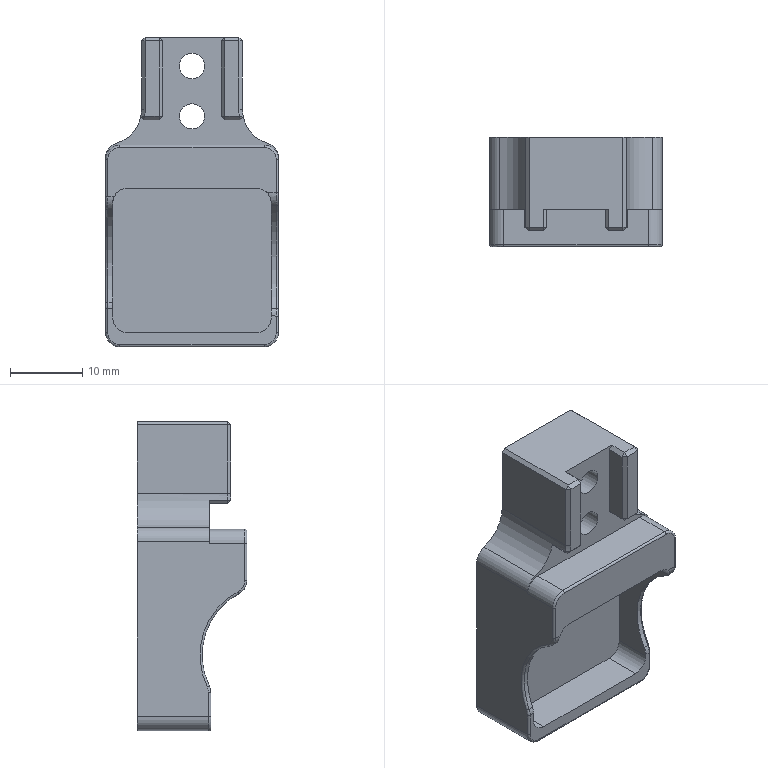CAM job | NX | 3+2 milling, drilling | part box 24 x 15.2 x 43 mm | stock box 25 x 20 x 48 mm
Tools:
number,name,description,diameter,corner_radius,flute_length,length,flutes
3,D3,平底铣刀-粗,3.0,0.0,20.0,75.0,2
6,D6,平底铣刀-粗,6.0,0.0,25.0,75.0,2
9,D10,平底铣刀-粗,10.0,0.0,35.0,75.0,2
17,D3-J,平底铣刀-精,3.0,0.0,50.0,75.0,2
11,D4-J,平底铣刀-精,4.0,0.0,50.0,75.0,2
10,D10-J,平底铣刀-精,10.0,0.0,35.0,75.0,2
1,D80R0.8飞刀,圆鼻刀-粗,80.0,0.8,50.0,75.0,2
2,D6倒角刀,倒角刀,6.0,0.0,3.0,25.0,2
18,R2,圆球刀,4.0,2.0,10.0,50.0,2
17,ZT3.5,钻头,3.5,0.0,35.0,50.0,2
Operations:
program,operation,operation_type,tool,method,geometry_group,spindle_rpm,surface_speed,feed_per_tooth,feed_cut,feed_plunge,cut_length_mm,path_length_mm,cut_time_min,machine_time_min
B,面铣自动飞面开粗一刀_COPY,FaceMilling,D80R0.8飞刀,分层开粗-切深K-步距G,W-B,4500.0,890.615,0.3333,3000.0,100.0,1359.0,2594.622,0.453,0.5766
B,面铣自动飞面精光一刀_COPY,FaceMilling,D80R0.8飞刀,侧刃精光-切深K-步距G,W-B,4500.0,890.615,0.1111,1000.0,100.0,151.0,187.0,0.151,0.1546
B,底壁铣分层开粗-中_COPY_1,VolumeBased25DMillingOperation,D6,分层开粗-切深K-步距G,W-B,8000.0,150.792,0.1875,3000.0,100.0,508.662,593.057,0.1696,0.178
B,型腔铣开粗-中_COPY,CavityMilling,D6,分层开粗-切深K-步距G,W-B,8000.0,150.792,0.1875,3000.0,100.0,6619.858,7262.06,2.207,2.298
B,底壁铣分层开粗-中_COPY,VolumeBased25DMillingOperation,D3,分层开粗-切深K-步距G,W-B,8000.0,100.528,0.125,2000.0,100.0,2179.609,2255.856,1.09,1.097
B,钻倒角_2_1,Operation,D6倒角刀,METHOD,W-B,8000.0,150.796,0.0625,1000.0,0.0,10.1,87.216,0.0101,0.0178
B,钻倒角_2,Operation,D6倒角刀,METHOD,W-B,8000.0,150.796,0.0625,1000.0,0.0,10.1,81.216,0.0101,0.0172
B,平面去毛刺6X45L_COPY,SurfaceContour,D6倒角刀,爬面_倒角-切深0-步距G,W-B,6500.0,122.519,0.1154,1500.0,100.0,80.316,288.414,0.0535,0.0744
B,平面去毛刺6X45L_COPY_1,SurfaceContour,D6倒角刀,爬面_倒角-切深0-步距G,W-B,6500.0,122.519,0.1154,1500.0,100.0,137.933,395.261,0.092,0.1177
B,等高精光往复爬面_COPY,ZLevelMilling,R2,等高爬面-切深K-步距G,W-B,7000.0,87.965,0.2857,4000.0,100.0,1484.177,1514.986,0.371,0.3741
B,等高精光往复爬面_COPY_COPY,ZLevelMilling,R2,等高爬面-切深K-步距G,W-B,7000.0,87.965,0.2857,4000.0,100.0,1338.431,1379.24,0.3346,0.3387
B,曲面D4R2,SurfaceContour,R2,METHOD,W-B,7000.0,87.965,0.25,3500.0,100.0,2277.059,2365.205,0.6506,0.6594
B,底壁铣精光底面-中_COPY,VolumeBased25DMillingOperation,D3-J,精光步距切深关,W-B,8000.0,100.528,0.05,800.0,100.0,89.951,228.14,0.1124,0.1263
B,底壁铣精光底面-中_COPY_3,VolumeBased25DMillingOperation,D3-J,精光步距切深关,W-B,7000.0,175.0,0.0536,1500.0,100.0,70.451,117.112,0.047,0.0516
B,底壁铣精光侧面-中-选底面_COPY,VolumeBased25DMillingOperation,D3-J,侧刃精光-切深K-步距G,W-B,8000.0,100.528,0.05,800.0,100.0,84.728,212.733,0.1059,0.1187
B,等高光顺清角D4参考10_COPY,ZLevelMilling,D4-J,分层精光-切深K-步距G,W-B,8000.0,100.528,0.0625,1000.0,100.0,1197.386,1332.303,1.197,1.211
B,底壁铣精光底面-中_COPY_2,VolumeBased25DMillingOperation,D4-J,精光步距切深关,W-B,7000.0,175.0,0.0536,1500.0,100.0,71.879,107.879,0.0479,0.0515
B,底壁铣精光底面-中_COPY_1,VolumeBased25DMillingOperation,D4-J,精光步距切深关,W-B,7000.0,175.0,0.0536,1500.0,100.0,178.594,224.494,0.1191,0.1237
B,底壁铣精光侧面-中-选底面_COPY_1,VolumeBased25DMillingOperation,D4-J,侧刃精光-切深K-步距G,W-B,8000.0,100.528,0.05,800.0,100.0,219.94,267.363,0.2749,0.2797
A,顶面,FaceMilling,D80R0.8飞刀,侧刃精光-切深K-步距G,W-A,4000.0,1005.31,0.125,1000.0,100.0,137.0,173.0,0.137,0.1406
A,外形粗_2,VolumeBased25DMillingOperation,D10,METHOD,W-A,8000.0,251.327,0.3125,5000.0,80.0,3482.346,3536.346,0.6965,0.7019
A,打点-深0.8,Operation,D6倒角刀,NONE,W-A,8000.0,150.796,0.0312,500.0,90.0,3.6,55.271,0.0072,0.0124
A,通孔-3-4,Operation,ZT3.5,NONE,W-A,3000.0,32.987,0.02,120.0,90.0,28.103,104.277,0.2342,0.2418
A,仅选体,SurfaceContour,D6倒角刀,METHOD,W-A,8000.0,150.796,0.1875,3000.0,100.0,142.237,177.438,0.0474,0.0509
A,钻倒角_1,Operation,D6倒角刀,METHOD,W-A,8000.0,150.796,0.0312,500.0,0.0,10.1,70.816,0.0202,0.0263
A,外形半精_2,VolumeBased25DMillingOperation,D10-J,METHOD,W-A,8000.0,251.327,0.0625,1000.0,100.0,162.611,232.611,0.1626,0.1696